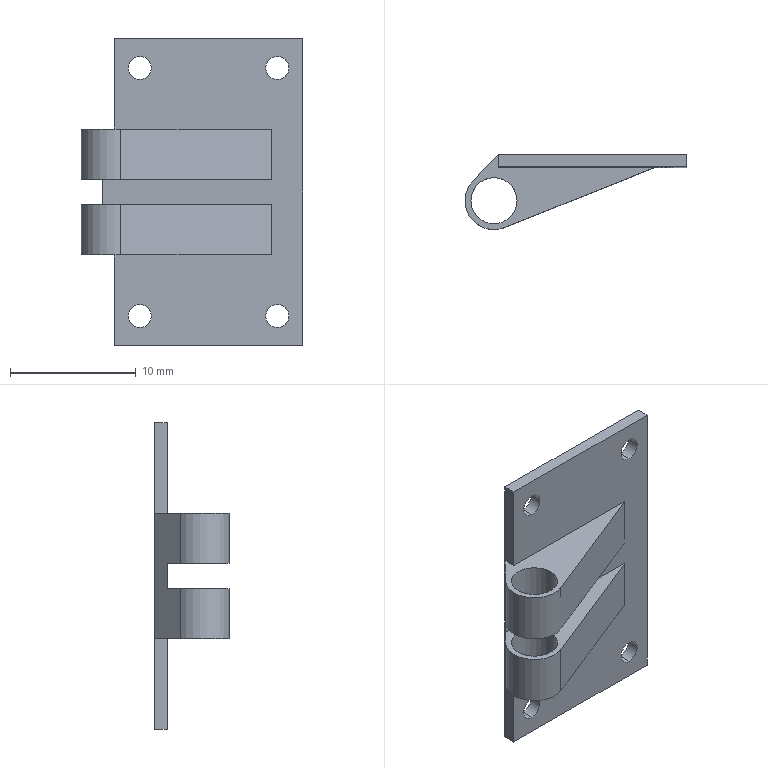Part | SolidWorks | features BaseBody 1 | 1 solid | 28 faces | box 17.607 x 5.957 x 24.289 mm | volume 605.772 mm3 | cylinder 14 | plane 14 | commonest cylinder face diameters 1.828 x8 3.663 x4 4.588 x2
STEP:
#1=CARTESIAN_POINT('',(185.615,42.862,-8.93));
#2=VERTEX_POINT('',#1);
#3=CARTESIAN_POINT('',(185.615,42.862,-10.758));
#4=VERTEX_POINT('',#3);
#5=CARTESIAN_POINT('',(185.615,42.862,-9.844));
#6=DIRECTION('',(0.,-1.,0.));
#7=DIRECTION('',(0.,0.,-1.));
#8=AXIS2_PLACEMENT_3D('',#5,#6,#7);
#9=CIRCLE('',#8,0.9139);
#10=EDGE_CURVE('',#2,#4,#9,.T.);
#11=ORIENTED_EDGE('',*,*,#10,.F.);
#12=CARTESIAN_POINT('',(185.615,41.862,-8.93));
#13=VERTEX_POINT('',#12);
#14=CARTESIAN_POINT('',(185.615,42.862,-8.93));
#15=DIRECTION('',(0.,-1.,0.));
#16=VECTOR('',#15,1000.);
#17=LINE('',#14,#16);
#18=EDGE_CURVE('',#2,#13,#17,.T.);
#19=ORIENTED_EDGE('',*,*,#18,.T.);
#20=CARTESIAN_POINT('',(185.615,41.862,-10.758));
#21=VERTEX_POINT('',#20);
#22=CARTESIAN_POINT('',(185.615,41.862,-9.844));
#23=DIRECTION('',(0.,1.,0.));
#24=DIRECTION('',(0.,0.,-1.));
#25=AXIS2_PLACEMENT_3D('',#22,#23,#24);
#26=CIRCLE('',#25,0.9139);
#27=EDGE_CURVE('',#21,#13,#26,.T.);
#28=ORIENTED_EDGE('',*,*,#27,.F.);
#29=CARTESIAN_POINT('',(185.615,42.862,-10.758));
#30=DIRECTION('',(0.,-1.,0.));
#31=VECTOR('',#30,1000.);
#32=LINE('',#29,#31);
#33=EDGE_CURVE('',#4,#21,#32,.T.);
#34=ORIENTED_EDGE('',*,*,#33,.F.);
#35=EDGE_LOOP('',(#11,#19,#28,#34));
#36=FACE_OUTER_BOUND('',#35,.T.);
#37=CARTESIAN_POINT('',(185.615,42.862,-9.844));
#38=DIRECTION('',(0.,-1.,0.));
#39=DIRECTION('',(0.,0.,-1.));
#40=AXIS2_PLACEMENT_3D('',#37,#38,#39);
#41=CYLINDRICAL_SURFACE('',#40,0.9139);
#42=ADVANCED_FACE('',(#36),#41,.F.);
#43=CARTESIAN_POINT('',(196.532,42.862,-8.93));
#44=VERTEX_POINT('',#43);
#45=CARTESIAN_POINT('',(196.532,42.862,-10.758));
#46=VERTEX_POINT('',#45);
#47=CARTESIAN_POINT('',(196.532,42.862,-9.844));
#48=DIRECTION('',(0.,-1.,0.));
#49=DIRECTION('',(0.,0.,-1.));
#50=AXIS2_PLACEMENT_3D('',#47,#48,#49);
#51=CIRCLE('',#50,0.9139);
#52=EDGE_CURVE('',#44,#46,#51,.T.);
#53=ORIENTED_EDGE('',*,*,#52,.F.);
#54=CARTESIAN_POINT('',(196.532,41.862,-8.93));
#55=VERTEX_POINT('',#54);
#56=CARTESIAN_POINT('',(196.532,42.862,-8.93));
#57=DIRECTION('',(0.,-1.,0.));
#58=VECTOR('',#57,1000.);
#59=LINE('',#56,#58);
#60=EDGE_CURVE('',#44,#55,#59,.T.);
#61=ORIENTED_EDGE('',*,*,#60,.T.);
#62=CARTESIAN_POINT('',(196.532,41.862,-10.758));
#63=VERTEX_POINT('',#62);
#64=CARTESIAN_POINT('',(196.532,41.862,-9.844));
#65=DIRECTION('',(0.,1.,0.));
#66=DIRECTION('',(0.,0.,-1.));
#67=AXIS2_PLACEMENT_3D('',#64,#65,#66);
#68=CIRCLE('',#67,0.9139);
#69=EDGE_CURVE('',#63,#55,#68,.T.);
#70=ORIENTED_EDGE('',*,*,#69,.F.);
#71=CARTESIAN_POINT('',(196.532,42.862,-10.758));
#72=DIRECTION('',(0.,-1.,0.));
#73=VECTOR('',#72,1000.);
#74=LINE('',#71,#73);
#75=EDGE_CURVE('',#46,#63,#74,.T.);
#76=ORIENTED_EDGE('',*,*,#75,.F.);
#77=EDGE_LOOP('',(#53,#61,#70,#76));
#78=FACE_OUTER_BOUND('',#77,.T.);
#79=CARTESIAN_POINT('',(196.532,42.862,-9.844));
#80=DIRECTION('',(0.,-1.,0.));
#81=DIRECTION('',(0.,0.,-1.));
#82=AXIS2_PLACEMENT_3D('',#79,#80,#81);
#83=CYLINDRICAL_SURFACE('',#82,0.9139);
#84=ADVANCED_FACE('',(#78),#83,.F.);
#85=CARTESIAN_POINT('',(196.532,42.862,10.758));
#86=VERTEX_POINT('',#85);
#87=CARTESIAN_POINT('',(196.532,42.862,8.93));
#88=VERTEX_POINT('',#87);
#89=CARTESIAN_POINT('',(196.532,42.862,9.844));
#90=DIRECTION('',(0.,-1.,0.));
#91=DIRECTION('',(0.,0.,-1.));
#92=AXIS2_PLACEMENT_3D('',#89,#90,#91);
#93=CIRCLE('',#92,0.9139);
#94=EDGE_CURVE('',#86,#88,#93,.T.);
#95=ORIENTED_EDGE('',*,*,#94,.F.);
#96=CARTESIAN_POINT('',(196.532,41.862,10.758));
#97=VERTEX_POINT('',#96);
#98=CARTESIAN_POINT('',(196.532,42.862,10.758));
#99=DIRECTION('',(0.,-1.,0.));
#100=VECTOR('',#99,1000.);
#101=LINE('',#98,#100);
#102=EDGE_CURVE('',#86,#97,#101,.T.);
#103=ORIENTED_EDGE('',*,*,#102,.T.);
#104=CARTESIAN_POINT('',(196.532,41.862,8.93));
#105=VERTEX_POINT('',#104);
#106=CARTESIAN_POINT('',(196.532,41.862,9.844));
#107=DIRECTION('',(0.,1.,0.));
#108=DIRECTION('',(0.,0.,-1.));
#109=AXIS2_PLACEMENT_3D('',#106,#107,#108);
#110=CIRCLE('',#109,0.9139);
#111=EDGE_CURVE('',#105,#97,#110,.T.);
#112=ORIENTED_EDGE('',*,*,#111,.F.);
#113=CARTESIAN_POINT('',(196.532,42.862,8.93));
#114=DIRECTION('',(0.,-1.,0.));
#115=VECTOR('',#114,1000.);
#116=LINE('',#113,#115);
#117=EDGE_CURVE('',#88,#105,#116,.T.);
#118=ORIENTED_EDGE('',*,*,#117,.F.);
#119=EDGE_LOOP('',(#95,#103,#112,#118));
#120=FACE_OUTER_BOUND('',#119,.T.);
#121=CARTESIAN_POINT('',(196.532,42.862,9.844));
#122=DIRECTION('',(0.,-1.,0.));
#123=DIRECTION('',(0.,0.,-1.));
#124=AXIS2_PLACEMENT_3D('',#121,#122,#123);
#125=CYLINDRICAL_SURFACE('',#124,0.9139);
#126=ADVANCED_FACE('',(#120),#125,.F.);
#127=CARTESIAN_POINT('',(185.615,42.862,10.758));
#128=VERTEX_POINT('',#127);
#129=CARTESIAN_POINT('',(185.615,42.862,8.93));
#130=VERTEX_POINT('',#129);
#131=CARTESIAN_POINT('',(185.615,42.862,9.844));
#132=DIRECTION('',(0.,-1.,0.));
#133=DIRECTION('',(0.,0.,-1.));
#134=AXIS2_PLACEMENT_3D('',#131,#132,#133);
#135=CIRCLE('',#134,0.9139);
#136=EDGE_CURVE('',#128,#130,#135,.T.);
#137=ORIENTED_EDGE('',*,*,#136,.F.);
#138=CARTESIAN_POINT('',(185.615,41.862,10.758));
#139=VERTEX_POINT('',#138);
#140=CARTESIAN_POINT('',(185.615,42.862,10.758));
#141=DIRECTION('',(0.,-1.,0.));
#142=VECTOR('',#141,1000.);
#143=LINE('',#140,#142);
#144=EDGE_CURVE('',#128,#139,#143,.T.);
#145=ORIENTED_EDGE('',*,*,#144,.T.);
#146=CARTESIAN_POINT('',(185.615,41.862,8.93));
#147=VERTEX_POINT('',#146);
#148=CARTESIAN_POINT('',(185.615,41.862,9.844));
#149=DIRECTION('',(0.,1.,0.));
#150=DIRECTION('',(0.,0.,-1.));
#151=AXIS2_PLACEMENT_3D('',#148,#149,#150);
#152=CIRCLE('',#151,0.9139);
#153=EDGE_CURVE('',#147,#139,#152,.T.);
#154=ORIENTED_EDGE('',*,*,#153,.F.);
#155=CARTESIAN_POINT('',(185.615,42.862,8.93));
#156=DIRECTION('',(0.,-1.,0.));
#157=VECTOR('',#156,1000.);
#158=LINE('',#155,#157);
#159=EDGE_CURVE('',#130,#147,#158,.T.);
#160=ORIENTED_EDGE('',*,*,#159,.F.);
#161=EDGE_LOOP('',(#137,#145,#154,#160));
#162=FACE_OUTER_BOUND('',#161,.T.);
#163=CARTESIAN_POINT('',(185.615,42.862,9.844));
#164=DIRECTION('',(0.,-1.,0.));
#165=DIRECTION('',(0.,0.,-1.));
#166=AXIS2_PLACEMENT_3D('',#163,#164,#165);
#167=CYLINDRICAL_SURFACE('',#166,0.9139);
#168=ADVANCED_FACE('',(#162),#167,.F.);
#169=CARTESIAN_POINT('',(185.074,39.199,-5.));
#170=VERTEX_POINT('',#169);
#171=CARTESIAN_POINT('',(181.411,39.199,-5.));
#172=VERTEX_POINT('',#171);
#173=CARTESIAN_POINT('',(183.243,39.199,-5.));
#174=DIRECTION('',(0.,0.,-1.));
#175=DIRECTION('',(1.,0.,0.));
#176=AXIS2_PLACEMENT_3D('',#173,#174,#175);
#177=CIRCLE('',#176,1.832);
#178=EDGE_CURVE('',#170,#172,#177,.T.);
#179=ORIENTED_EDGE('',*,*,#178,.T.);
#180=CARTESIAN_POINT('',(181.411,39.199,-1.));
#181=VERTEX_POINT('',#180);
#182=CARTESIAN_POINT('',(181.411,39.199,0.));
#183=DIRECTION('',(0.,0.,1.));
#184=VECTOR('',#183,1000.);
#185=LINE('',#182,#184);
#186=EDGE_CURVE('',#172,#181,#185,.T.);
#187=ORIENTED_EDGE('',*,*,#186,.T.);
#188=CARTESIAN_POINT('',(185.074,39.199,-1.));
#189=VERTEX_POINT('',#188);
#190=CARTESIAN_POINT('',(183.243,39.199,-1.));
#191=DIRECTION('',(0.,0.,1.));
#192=DIRECTION('',(1.,0.,0.));
#193=AXIS2_PLACEMENT_3D('',#190,#191,#192);
#194=CIRCLE('',#193,1.832);
#195=EDGE_CURVE('',#181,#189,#194,.T.);
#196=ORIENTED_EDGE('',*,*,#195,.T.);
#197=CARTESIAN_POINT('',(185.074,39.199,0.));
#198=DIRECTION('',(0.,0.,1.));
#199=VECTOR('',#198,1000.);
#200=LINE('',#197,#199);
#201=EDGE_CURVE('',#170,#189,#200,.T.);
#202=ORIENTED_EDGE('',*,*,#201,.F.);
#203=EDGE_LOOP('',(#179,#187,#196,#202));
#204=FACE_OUTER_BOUND('',#203,.T.);
#205=CARTESIAN_POINT('',(183.243,39.199,0.));
#206=DIRECTION('',(0.,0.,1.));
#207=DIRECTION('',(1.,0.,0.));
#208=AXIS2_PLACEMENT_3D('',#205,#206,#207);
#209=CYLINDRICAL_SURFACE('',#208,1.832);
#210=ADVANCED_FACE('',(#204),#209,.F.);
#211=CARTESIAN_POINT('',(185.074,39.199,1.));
#212=VERTEX_POINT('',#211);
#213=CARTESIAN_POINT('',(181.411,39.199,1.));
#214=VERTEX_POINT('',#213);
#215=CARTESIAN_POINT('',(183.243,39.199,1.));
#216=DIRECTION('',(0.,0.,-1.));
#217=DIRECTION('',(1.,0.,0.));
#218=AXIS2_PLACEMENT_3D('',#215,#216,#217);
#219=CIRCLE('',#218,1.832);
#220=EDGE_CURVE('',#212,#214,#219,.T.);
#221=ORIENTED_EDGE('',*,*,#220,.T.);
#222=CARTESIAN_POINT('',(181.411,39.199,5.));
#223=VERTEX_POINT('',#222);
#224=CARTESIAN_POINT('',(181.411,39.199,0.));
#225=DIRECTION('',(0.,0.,1.));
#226=VECTOR('',#225,1000.);
#227=LINE('',#224,#226);
#228=EDGE_CURVE('',#214,#223,#227,.T.);
#229=ORIENTED_EDGE('',*,*,#228,.T.);
#230=CARTESIAN_POINT('',(185.074,39.199,5.));
#231=VERTEX_POINT('',#230);
#232=CARTESIAN_POINT('',(183.243,39.199,5.));
#233=DIRECTION('',(0.,0.,-1.));
#234=DIRECTION('',(1.,0.,0.));
#235=AXIS2_PLACEMENT_3D('',#232,#233,#234);
#236=CIRCLE('',#235,1.832);
#237=EDGE_CURVE('',#231,#223,#236,.T.);
#238=ORIENTED_EDGE('',*,*,#237,.F.);
#239=CARTESIAN_POINT('',(185.074,39.199,0.));
#240=DIRECTION('',(0.,0.,1.));
#241=VECTOR('',#240,1000.);
#242=LINE('',#239,#241);
#243=EDGE_CURVE('',#212,#231,#242,.T.);
#244=ORIENTED_EDGE('',*,*,#243,.F.);
#245=EDGE_LOOP('',(#221,#229,#238,#244));
#246=FACE_OUTER_BOUND('',#245,.T.);
#247=CARTESIAN_POINT('',(183.243,39.199,0.));
#248=DIRECTION('',(0.,0.,1.));
#249=DIRECTION('',(1.,0.,0.));
#250=AXIS2_PLACEMENT_3D('',#247,#248,#249);
#251=CYLINDRICAL_SURFACE('',#250,1.832);
#252=ADVANCED_FACE('',(#246),#251,.F.);
#253=CARTESIAN_POINT('',(185.615,42.862,-9.844));
#254=DIRECTION('',(0.,-1.,0.));
#255=DIRECTION('',(0.,0.,-1.));
#256=AXIS2_PLACEMENT_3D('',#253,#254,#255);
#257=CIRCLE('',#256,0.9139);
#258=EDGE_CURVE('',#4,#2,#257,.T.);
#259=ORIENTED_EDGE('',*,*,#258,.T.);
#260=ORIENTED_EDGE('',*,*,#10,.T.);
#261=EDGE_LOOP('',(#259,#260));
#262=FACE_BOUND('',#261,.T.);
#263=CARTESIAN_POINT('',(196.532,42.862,-9.844));
#264=DIRECTION('',(0.,-1.,0.));
#265=DIRECTION('',(0.,0.,-1.));
#266=AXIS2_PLACEMENT_3D('',#263,#264,#265);
#267=CIRCLE('',#266,0.9139);
#268=EDGE_CURVE('',#46,#44,#267,.T.);
#269=ORIENTED_EDGE('',*,*,#268,.T.);
#270=ORIENTED_EDGE('',*,*,#52,.T.);
#271=EDGE_LOOP('',(#269,#270));
#272=FACE_BOUND('',#271,.T.);
#273=CARTESIAN_POINT('',(196.532,42.862,9.844));
#274=DIRECTION('',(0.,-1.,0.));
#275=DIRECTION('',(0.,0.,-1.));
#276=AXIS2_PLACEMENT_3D('',#273,#274,#275);
#277=CIRCLE('',#276,0.9139);
#278=EDGE_CURVE('',#88,#86,#277,.T.);
#279=ORIENTED_EDGE('',*,*,#278,.T.);
#280=ORIENTED_EDGE('',*,*,#94,.T.);
#281=EDGE_LOOP('',(#279,#280));
#282=FACE_BOUND('',#281,.T.);
#283=CARTESIAN_POINT('',(185.615,42.862,9.844));
#284=DIRECTION('',(0.,-1.,0.));
#285=DIRECTION('',(0.,0.,-1.));
#286=AXIS2_PLACEMENT_3D('',#283,#284,#285);
#287=CIRCLE('',#286,0.9139);
#288=EDGE_CURVE('',#130,#128,#287,.T.);
#289=ORIENTED_EDGE('',*,*,#288,.T.);
#290=ORIENTED_EDGE('',*,*,#136,.T.);
#291=EDGE_LOOP('',(#289,#290));
#292=FACE_BOUND('',#291,.T.);
#293=CARTESIAN_POINT('',(198.556,42.862,-12.144));
#294=VERTEX_POINT('',#293);
#295=CARTESIAN_POINT('',(183.591,42.862,-12.144));
#296=VERTEX_POINT('',#295);
#297=CARTESIAN_POINT('',(198.556,42.862,-12.144));
#298=DIRECTION('',(-1.,0.,0.));
#299=VECTOR('',#298,1000.);
#300=LINE('',#297,#299);
#301=EDGE_CURVE('',#294,#296,#300,.T.);
#302=ORIENTED_EDGE('',*,*,#301,.T.);
#303=CARTESIAN_POINT('',(183.591,42.862,-5.));
#304=VERTEX_POINT('',#303);
#305=CARTESIAN_POINT('',(183.591,42.862,0.));
#306=DIRECTION('',(0.,0.,1.));
#307=VECTOR('',#306,1000.);
#308=LINE('',#305,#307);
#309=EDGE_CURVE('',#296,#304,#308,.T.);
#310=ORIENTED_EDGE('',*,*,#309,.T.);
#311=CARTESIAN_POINT('',(183.591,42.862,5.));
#312=VERTEX_POINT('',#311);
#313=CARTESIAN_POINT('',(183.591,42.862,0.));
#314=DIRECTION('',(0.,0.,1.));
#315=VECTOR('',#314,1000.);
#316=LINE('',#313,#315);
#317=EDGE_CURVE('',#304,#312,#316,.T.);
#318=ORIENTED_EDGE('',*,*,#317,.T.);
#319=CARTESIAN_POINT('',(183.591,42.862,12.144));
#320=VERTEX_POINT('',#319);
#321=CARTESIAN_POINT('',(183.591,42.862,0.));
#322=DIRECTION('',(0.,0.,1.));
#323=VECTOR('',#322,1000.);
#324=LINE('',#321,#323);
#325=EDGE_CURVE('',#312,#320,#324,.T.);
#326=ORIENTED_EDGE('',*,*,#325,.T.);
#327=CARTESIAN_POINT('',(198.556,42.862,12.144));
#328=VERTEX_POINT('',#327);
#329=CARTESIAN_POINT('',(198.556,42.862,12.144));
#330=DIRECTION('',(1.,0.,0.));
#331=VECTOR('',#330,1000.);
#332=LINE('',#329,#331);
#333=EDGE_CURVE('',#320,#328,#332,.T.);
#334=ORIENTED_EDGE('',*,*,#333,.T.);
#335=CARTESIAN_POINT('',(198.556,42.862,0.));
#336=DIRECTION('',(0.,0.,-1.));
#337=VECTOR('',#336,1000.);
#338=LINE('',#335,#337);
#339=EDGE_CURVE('',#328,#294,#338,.T.);
#340=ORIENTED_EDGE('',*,*,#339,.T.);
#341=EDGE_LOOP('',(#302,#310,#318,#326,#334,#340));
#342=FACE_OUTER_BOUND('',#341,.T.);
#343=CARTESIAN_POINT('',(198.556,42.862,0.));
#344=DIRECTION('',(0.,1.,0.));
#345=DIRECTION('',(0.,0.,1.));
#346=AXIS2_PLACEMENT_3D('',#343,#344,#345);
#347=PLANE('',#346);
#348=ADVANCED_FACE('',(#262,#272,#282,#292,#342),#347,.T.);
#349=ORIENTED_EDGE('',*,*,#18,.F.);
#350=ORIENTED_EDGE('',*,*,#258,.F.);
#351=ORIENTED_EDGE('',*,*,#33,.T.);
#352=CARTESIAN_POINT('',(185.615,41.862,-9.844));
#353=DIRECTION('',(0.,1.,0.));
#354=DIRECTION('',(0.,0.,-1.));
#355=AXIS2_PLACEMENT_3D('',#352,#353,#354);
#356=CIRCLE('',#355,0.9139);
#357=EDGE_CURVE('',#13,#21,#356,.T.);
#358=ORIENTED_EDGE('',*,*,#357,.F.);
#359=EDGE_LOOP('',(#349,#350,#351,#358));
#360=FACE_OUTER_BOUND('',#359,.T.);
#361=CARTESIAN_POINT('',(185.615,42.862,-9.844));
#362=DIRECTION('',(0.,-1.,0.));
#363=DIRECTION('',(0.,0.,-1.));
#364=AXIS2_PLACEMENT_3D('',#361,#362,#363);
#365=CYLINDRICAL_SURFACE('',#364,0.9139);
#366=ADVANCED_FACE('',(#360),#365,.F.);
#367=ORIENTED_EDGE('',*,*,#60,.F.);
#368=ORIENTED_EDGE('',*,*,#268,.F.);
#369=ORIENTED_EDGE('',*,*,#75,.T.);
#370=CARTESIAN_POINT('',(196.532,41.862,-9.844));
#371=DIRECTION('',(0.,1.,0.));
#372=DIRECTION('',(0.,0.,-1.));
#373=AXIS2_PLACEMENT_3D('',#370,#371,#372);
#374=CIRCLE('',#373,0.9139);
#375=EDGE_CURVE('',#55,#63,#374,.T.);
#376=ORIENTED_EDGE('',*,*,#375,.F.);
#377=EDGE_LOOP('',(#367,#368,#369,#376));
#378=FACE_OUTER_BOUND('',#377,.T.);
#379=CARTESIAN_POINT('',(196.532,42.862,-9.844));
#380=DIRECTION('',(0.,-1.,0.));
#381=DIRECTION('',(0.,0.,-1.));
#382=AXIS2_PLACEMENT_3D('',#379,#380,#381);
#383=CYLINDRICAL_SURFACE('',#382,0.9139);
#384=ADVANCED_FACE('',(#378),#383,.F.);
#385=ORIENTED_EDGE('',*,*,#102,.F.);
#386=ORIENTED_EDGE('',*,*,#278,.F.);
#387=ORIENTED_EDGE('',*,*,#117,.T.);
#388=CARTESIAN_POINT('',(196.532,41.862,9.844));
#389=DIRECTION('',(0.,1.,0.));
#390=DIRECTION('',(0.,0.,-1.));
#391=AXIS2_PLACEMENT_3D('',#388,#389,#390);
#392=CIRCLE('',#391,0.9139);
#393=EDGE_CURVE('',#97,#105,#392,.T.);
#394=ORIENTED_EDGE('',*,*,#393,.F.);
#395=EDGE_LOOP('',(#385,#386,#387,#394));
#396=FACE_OUTER_BOUND('',#395,.T.);
#397=CARTESIAN_POINT('',(196.532,42.862,9.844));
#398=DIRECTION('',(0.,-1.,0.));
#399=DIRECTION('',(0.,0.,-1.));
#400=AXIS2_PLACEMENT_3D('',#397,#398,#399);
#401=CYLINDRICAL_SURFACE('',#400,0.9139);
#402=ADVANCED_FACE('',(#396),#401,.F.);
#403=ORIENTED_EDGE('',*,*,#144,.F.);
#404=ORIENTED_EDGE('',*,*,#288,.F.);
#405=ORIENTED_EDGE('',*,*,#159,.T.);
#406=CARTESIAN_POINT('',(185.615,41.862,9.844));
#407=DIRECTION('',(0.,1.,0.));
#408=DIRECTION('',(0.,0.,-1.));
#409=AXIS2_PLACEMENT_3D('',#406,#407,#408);
#410=CIRCLE('',#409,0.9139);
#411=EDGE_CURVE('',#139,#147,#410,.T.);
#412=ORIENTED_EDGE('',*,*,#411,.F.);
#413=EDGE_LOOP('',(#403,#404,#405,#412));
#414=FACE_OUTER_BOUND('',#413,.T.);
#415=CARTESIAN_POINT('',(185.615,42.862,9.844));
#416=DIRECTION('',(0.,-1.,0.));
#417=DIRECTION('',(0.,0.,-1.));
#418=AXIS2_PLACEMENT_3D('',#415,#416,#417);
#419=CYLINDRICAL_SURFACE('',#418,0.9139);
#420=ADVANCED_FACE('',(#414),#419,.F.);
#421=CARTESIAN_POINT('',(183.591,41.862,-12.144));
#422=VERTEX_POINT('',#421);
#423=CARTESIAN_POINT('',(183.591,42.862,-12.144));
#424=DIRECTION('',(0.,-1.,0.));
#425=VECTOR('',#424,1000.);
#426=LINE('',#423,#425);
#427=EDGE_CURVE('',#296,#422,#426,.T.);
#428=ORIENTED_EDGE('',*,*,#427,.T.);
#429=CARTESIAN_POINT('',(183.591,41.862,-5.));
#430=VERTEX_POINT('',#429);
#431=CARTESIAN_POINT('',(183.591,41.862,12.144));
#432=DIRECTION('',(0.,0.,1.));
#433=VECTOR('',#432,1000.);
#434=LINE('',#431,#433);
#435=EDGE_CURVE('',#422,#430,#434,.T.);
#436=ORIENTED_EDGE('',*,*,#435,.T.);
#437=CARTESIAN_POINT('',(183.591,39.884,-5.));
#438=DIRECTION('',(0.,1.,0.));
#439=VECTOR('',#438,1000.);
#440=LINE('',#437,#439);
#441=EDGE_CURVE('',#430,#304,#440,.T.);
#442=ORIENTED_EDGE('',*,*,#441,.T.);
#443=ORIENTED_EDGE('',*,*,#309,.F.);
#444=EDGE_LOOP('',(#428,#436,#442,#443));
#445=FACE_OUTER_BOUND('',#444,.T.);
#446=CARTESIAN_POINT('',(183.591,42.862,12.144));
#447=DIRECTION('',(-1.,0.,0.));
#448=DIRECTION('',(0.,0.,1.));
#449=AXIS2_PLACEMENT_3D('',#446,#447,#448);
#450=PLANE('',#449);
#451=ADVANCED_FACE('',(#445),#450,.T.);
#452=CARTESIAN_POINT('',(198.556,41.862,-12.144));
#453=VERTEX_POINT('',#452);
#454=CARTESIAN_POINT('',(183.591,41.862,-12.144));
#455=DIRECTION('',(-1.,0.,0.));
#456=VECTOR('',#455,1000.);
#457=LINE('',#454,#456);
#458=EDGE_CURVE('',#453,#422,#457,.T.);
#459=ORIENTED_EDGE('',*,*,#458,.T.);
#460=ORIENTED_EDGE('',*,*,#427,.F.);
#461=ORIENTED_EDGE('',*,*,#301,.F.);
#462=CARTESIAN_POINT('',(198.556,42.862,-12.144));
#463=DIRECTION('',(0.,-1.,0.));
#464=VECTOR('',#463,1000.);
#465=LINE('',#462,#464);
#466=EDGE_CURVE('',#294,#453,#465,.T.);
#467=ORIENTED_EDGE('',*,*,#466,.T.);
#468=EDGE_LOOP('',(#459,#460,#461,#467));
#469=FACE_OUTER_BOUND('',#468,.T.);
#470=CARTESIAN_POINT('',(183.591,42.862,-12.144));
#471=DIRECTION('',(0.,0.,-1.));
#472=DIRECTION('',(-1.,0.,0.));
#473=AXIS2_PLACEMENT_3D('',#470,#471,#472);
#474=PLANE('',#473);
#475=ADVANCED_FACE('',(#469),#474,.T.);
#476=CARTESIAN_POINT('',(198.556,41.862,12.144));
#477=VERTEX_POINT('',#476);
#478=CARTESIAN_POINT('',(198.556,41.862,-12.144));
#479=DIRECTION('',(0.,0.,-1.));
#480=VECTOR('',#479,1000.);
#481=LINE('',#478,#480);
#482=EDGE_CURVE('',#477,#453,#481,.T.);
#483=ORIENTED_EDGE('',*,*,#482,.T.);
#484=ORIENTED_EDGE('',*,*,#466,.F.);
#485=ORIENTED_EDGE('',*,*,#339,.F.);
#486=CARTESIAN_POINT('',(198.556,42.862,12.144));
#487=DIRECTION('',(0.,-1.,0.));
#488=VECTOR('',#487,1000.);
#489=LINE('',#486,#488);
#490=EDGE_CURVE('',#328,#477,#489,.T.);
#491=ORIENTED_EDGE('',*,*,#490,.T.);
#492=EDGE_LOOP('',(#483,#484,#485,#491));
#493=FACE_OUTER_BOUND('',#492,.T.);
#494=CARTESIAN_POINT('',(198.556,42.862,-12.144));
#495=DIRECTION('',(1.,0.,0.));
#496=DIRECTION('',(0.,0.,-1.));
#497=AXIS2_PLACEMENT_3D('',#494,#495,#496);
#498=PLANE('',#497);
#499=ADVANCED_FACE('',(#493),#498,.T.);
#500=CARTESIAN_POINT('',(183.591,41.862,12.144));
#501=VERTEX_POINT('',#500);
#502=CARTESIAN_POINT('',(198.556,41.862,12.144));
#503=DIRECTION('',(1.,0.,0.));
#504=VECTOR('',#503,1000.);
#505=LINE('',#502,#504);
#506=EDGE_CURVE('',#501,#477,#505,.T.);
#507=ORIENTED_EDGE('',*,*,#506,.T.);
#508=ORIENTED_EDGE('',*,*,#490,.F.);
#509=ORIENTED_EDGE('',*,*,#333,.F.);
#510=CARTESIAN_POINT('',(183.591,42.862,12.144));
#511=DIRECTION('',(0.,-1.,0.));
#512=VECTOR('',#511,1000.);
#513=LINE('',#510,#512);
#514=EDGE_CURVE('',#320,#501,#513,.T.);
#515=ORIENTED_EDGE('',*,*,#514,.T.);
#516=EDGE_LOOP('',(#507,#508,#509,#515));
#517=FACE_OUTER_BOUND('',#516,.T.);
#518=CARTESIAN_POINT('',(198.556,42.862,12.144));
#519=DIRECTION('',(0.,0.,1.));
#520=DIRECTION('',(1.,0.,0.));
#521=AXIS2_PLACEMENT_3D('',#518,#519,#520);
#522=PLANE('',#521);
#523=ADVANCED_FACE('',(#517),#522,.T.);
#524=ORIENTED_EDGE('',*,*,#514,.F.);
#525=ORIENTED_EDGE('',*,*,#325,.F.);
#526=CARTESIAN_POINT('',(183.591,41.862,5.));
#527=VERTEX_POINT('',#526);
#528=CARTESIAN_POINT('',(183.591,39.884,5.));
#529=DIRECTION('',(0.,1.,0.));
#530=VECTOR('',#529,1000.);
#531=LINE('',#528,#530);
#532=EDGE_CURVE('',#527,#312,#531,.T.);
#533=ORIENTED_EDGE('',*,*,#532,.F.);
#534=CARTESIAN_POINT('',(183.591,41.862,12.144));
#535=DIRECTION('',(0.,0.,1.));
#536=VECTOR('',#535,1000.);
#537=LINE('',#534,#536);
#538=EDGE_CURVE('',#527,#501,#537,.T.);
#539=ORIENTED_EDGE('',*,*,#538,.T.);
#540=EDGE_LOOP('',(#524,#525,#533,#539));
#541=FACE_OUTER_BOUND('',#540,.T.);
#542=CARTESIAN_POINT('',(183.591,42.862,12.144));
#543=DIRECTION('',(-1.,0.,0.));
#544=DIRECTION('',(0.,0.,1.));
#545=AXIS2_PLACEMENT_3D('',#542,#543,#544);
#546=PLANE('',#545);
#547=ADVANCED_FACE('',(#541),#546,.T.);
#548=CARTESIAN_POINT('',(181.592,40.793,-5.));
#549=VERTEX_POINT('',#548);
#550=CARTESIAN_POINT('',(183.591,42.862,-5.));
#551=DIRECTION('',(-0.6946,-0.7194,0.));
#552=VECTOR('',#551,1000.);
#553=LINE('',#550,#552);
#554=EDGE_CURVE('',#304,#549,#553,.T.);
#555=ORIENTED_EDGE('',*,*,#554,.T.);
#556=CARTESIAN_POINT('',(181.592,40.793,-1.));
#557=VERTEX_POINT('',#556);
#558=CARTESIAN_POINT('',(181.592,40.793,0.));
#559=DIRECTION('',(0.,0.,1.));
#560=VECTOR('',#559,1000.);
#561=LINE('',#558,#560);
#562=EDGE_CURVE('',#549,#557,#561,.T.);
#563=ORIENTED_EDGE('',*,*,#562,.T.);
#564=CARTESIAN_POINT('',(182.626,41.863,-1.));
#565=VERTEX_POINT('',#564);
#566=CARTESIAN_POINT('',(181.592,40.793,-1.));
#567=DIRECTION('',(0.6946,0.7194,0.));
#568=VECTOR('',#567,1000.);
#569=LINE('',#566,#568);
#570=EDGE_CURVE('',#557,#565,#569,.T.);
#571=ORIENTED_EDGE('',*,*,#570,.T.);
#572=CARTESIAN_POINT('',(182.626,41.862,1.));
#573=VERTEX_POINT('',#572);
#574=CARTESIAN_POINT('',(182.626,41.863,0.));
#575=DIRECTION('',(0.,0.,1.));
#576=VECTOR('',#575,1000.);
#577=LINE('',#574,#576);
#578=EDGE_CURVE('',#565,#573,#577,.T.);
#579=ORIENTED_EDGE('',*,*,#578,.T.);
#580=CARTESIAN_POINT('',(181.592,40.793,1.));
#581=VERTEX_POINT('',#580);
#582=CARTESIAN_POINT('',(182.626,41.862,1.));
#583=DIRECTION('',(-0.6946,-0.7194,0.));
#584=VECTOR('',#583,1000.);
#585=LINE('',#582,#584);
#586=EDGE_CURVE('',#573,#581,#585,.T.);
#587=ORIENTED_EDGE('',*,*,#586,.T.);
#588=CARTESIAN_POINT('',(181.592,40.793,5.));
#589=VERTEX_POINT('',#588);
#590=CARTESIAN_POINT('',(181.592,40.793,0.));
#591=DIRECTION('',(0.,0.,1.));
#592=VECTOR('',#591,1000.);
#593=LINE('',#590,#592);
#594=EDGE_CURVE('',#581,#589,#593,.T.);
#595=ORIENTED_EDGE('',*,*,#594,.T.);
#596=CARTESIAN_POINT('',(183.591,42.862,5.));
#597=DIRECTION('',(0.6946,0.7194,0.));
#598=VECTOR('',#597,1000.);
#599=LINE('',#596,#598);
#600=EDGE_CURVE('',#589,#312,#599,.T.);
#601=ORIENTED_EDGE('',*,*,#600,.T.);
#602=ORIENTED_EDGE('',*,*,#317,.F.);
#603=EDGE_LOOP('',(#555,#563,#571,#579,#587,#595,#601,#602));
#604=FACE_OUTER_BOUND('',#603,.T.);
#605=CARTESIAN_POINT('',(183.591,42.862,0.));
#606=DIRECTION('',(-0.7194,0.6946,0.));
#607=DIRECTION('',(-0.6946,-0.7194,0.));
#608=AXIS2_PLACEMENT_3D('',#605,#606,#607);
#609=PLANE('',#608);
#610=ADVANCED_FACE('',(#604),#609,.T.);
#611=ORIENTED_EDGE('',*,*,#27,.T.);
#612=ORIENTED_EDGE('',*,*,#357,.T.);
#613=EDGE_LOOP('',(#611,#612));
#614=FACE_BOUND('',#613,.T.);
#615=ORIENTED_EDGE('',*,*,#69,.T.);
#616=ORIENTED_EDGE('',*,*,#375,.T.);
#617=EDGE_LOOP('',(#615,#616));
#618=FACE_BOUND('',#617,.T.);
#619=ORIENTED_EDGE('',*,*,#111,.T.);
#620=ORIENTED_EDGE('',*,*,#393,.T.);
#621=EDGE_LOOP('',(#619,#620));
#622=FACE_BOUND('',#621,.T.);
#623=ORIENTED_EDGE('',*,*,#153,.T.);
#624=ORIENTED_EDGE('',*,*,#411,.T.);
#625=EDGE_LOOP('',(#623,#624));
#626=FACE_BOUND('',#625,.T.);
#627=CARTESIAN_POINT('',(196.06,41.862,-5.));
#628=VERTEX_POINT('',#627);
#629=CARTESIAN_POINT('',(191.074,41.862,-5.));
#630=DIRECTION('',(1.,0.,0.));
#631=VECTOR('',#630,1000.);
#632=LINE('',#629,#631);
#633=EDGE_CURVE('',#430,#628,#632,.T.);
#634=ORIENTED_EDGE('',*,*,#633,.F.);
#635=ORIENTED_EDGE('',*,*,#435,.F.);
#636=ORIENTED_EDGE('',*,*,#458,.F.);
#637=ORIENTED_EDGE('',*,*,#482,.F.);
#638=ORIENTED_EDGE('',*,*,#506,.F.);
#639=ORIENTED_EDGE('',*,*,#538,.F.);
#640=CARTESIAN_POINT('',(196.06,41.862,5.));
#641=VERTEX_POINT('',#640);
#642=CARTESIAN_POINT('',(191.074,41.862,5.));
#643=DIRECTION('',(-1.,0.,0.));
#644=VECTOR('',#643,1000.);
#645=LINE('',#642,#644);
#646=EDGE_CURVE('',#641,#527,#645,.T.);
#647=ORIENTED_EDGE('',*,*,#646,.F.);
#648=CARTESIAN_POINT('',(196.06,41.862,1.));
#649=VERTEX_POINT('',#648);
#650=CARTESIAN_POINT('',(196.06,41.862,0.));
#651=DIRECTION('',(0.,0.,1.));
#652=VECTOR('',#651,1000.);
#653=LINE('',#650,#652);
#654=EDGE_CURVE('',#649,#641,#653,.T.);
#655=ORIENTED_EDGE('',*,*,#654,.F.);
#656=CARTESIAN_POINT('',(191.074,41.862,1.));
#657=DIRECTION('',(1.,0.,0.));
#658=VECTOR('',#657,1000.);
#659=LINE('',#656,#658);
#660=EDGE_CURVE('',#573,#649,#659,.T.);
#661=ORIENTED_EDGE('',*,*,#660,.F.);
#662=ORIENTED_EDGE('',*,*,#578,.F.);
#663=CARTESIAN_POINT('',(196.06,41.862,-1.));
#664=VERTEX_POINT('',#663);
#665=CARTESIAN_POINT('',(191.074,41.862,-1.));
#666=DIRECTION('',(-1.,0.,0.));
#667=VECTOR('',#666,1000.);
#668=LINE('',#665,#667);
#669=EDGE_CURVE('',#664,#565,#668,.T.);
#670=ORIENTED_EDGE('',*,*,#669,.F.);
#671=CARTESIAN_POINT('',(196.06,41.862,0.));
#672=DIRECTION('',(0.,0.,1.));
#673=VECTOR('',#672,1000.);
#674=LINE('',#671,#673);
#675=EDGE_CURVE('',#628,#664,#674,.T.);
#676=ORIENTED_EDGE('',*,*,#675,.F.);
#677=EDGE_LOOP('',(#634,#635,#636,#637,#638,#639,#647,#655,#661,#662,#670,#676));
#678=FACE_OUTER_BOUND('',#677,.T.);
#679=CARTESIAN_POINT('',(191.074,41.862,0.));
#680=DIRECTION('',(0.,1.,0.));
#681=DIRECTION('',(0.,0.,1.));
#682=AXIS2_PLACEMENT_3D('',#679,#680,#681);
#683=PLANE('',#682);
#684=ADVANCED_FACE('',(#614,#618,#622,#626,#678),#683,.F.);
#685=CARTESIAN_POINT('',(184.096,37.07,-5.));
#686=VERTEX_POINT('',#685);
#687=CARTESIAN_POINT('',(183.243,39.199,-5.));
#688=DIRECTION('',(0.,0.,1.));
#689=DIRECTION('',(1.,0.,0.));
#690=AXIS2_PLACEMENT_3D('',#687,#688,#689);
#691=CIRCLE('',#690,2.294);
#692=EDGE_CURVE('',#549,#686,#691,.T.);
#693=ORIENTED_EDGE('',*,*,#692,.T.);
#694=CARTESIAN_POINT('',(184.096,37.07,-1.));
#695=VERTEX_POINT('',#694);
#696=CARTESIAN_POINT('',(184.096,37.07,0.));
#697=DIRECTION('',(0.,0.,1.));
#698=VECTOR('',#697,1000.);
#699=LINE('',#696,#698);
#700=EDGE_CURVE('',#686,#695,#699,.T.);
#701=ORIENTED_EDGE('',*,*,#700,.T.);
#702=CARTESIAN_POINT('',(183.243,39.199,-1.));
#703=DIRECTION('',(0.,0.,-1.));
#704=DIRECTION('',(1.,0.,0.));
#705=AXIS2_PLACEMENT_3D('',#702,#703,#704);
#706=CIRCLE('',#705,2.294);
#707=EDGE_CURVE('',#695,#557,#706,.T.);
#708=ORIENTED_EDGE('',*,*,#707,.T.);
#709=ORIENTED_EDGE('',*,*,#562,.F.);
#710=EDGE_LOOP('',(#693,#701,#708,#709));
#711=FACE_OUTER_BOUND('',#710,.T.);
#712=CARTESIAN_POINT('',(183.243,39.199,0.));
#713=DIRECTION('',(0.,0.,1.));
#714=DIRECTION('',(1.,0.,0.));
#715=AXIS2_PLACEMENT_3D('',#712,#713,#714);
#716=CYLINDRICAL_SURFACE('',#715,2.294);
#717=ADVANCED_FACE('',(#711),#716,.T.);
#718=ORIENTED_EDGE('',*,*,#178,.F.);
#719=CARTESIAN_POINT('',(183.243,39.199,-5.));
#720=DIRECTION('',(0.,0.,-1.));
#721=DIRECTION('',(1.,0.,0.));
#722=AXIS2_PLACEMENT_3D('',#719,#720,#721);
#723=CIRCLE('',#722,1.832);
#724=EDGE_CURVE('',#172,#170,#723,.T.);
#725=ORIENTED_EDGE('',*,*,#724,.F.);
#726=EDGE_LOOP('',(#718,#725));
#727=FACE_BOUND('',#726,.T.);
#728=CARTESIAN_POINT('',(184.096,37.07,-5.));
#729=DIRECTION('',(0.9283,0.3719,0.));
#730=VECTOR('',#729,1000.);
#731=LINE('',#728,#730);
#732=EDGE_CURVE('',#686,#628,#731,.T.);
#733=ORIENTED_EDGE('',*,*,#732,.F.);
#734=ORIENTED_EDGE('',*,*,#692,.F.);
#735=ORIENTED_EDGE('',*,*,#554,.F.);
#736=ORIENTED_EDGE('',*,*,#441,.F.);
#737=ORIENTED_EDGE('',*,*,#633,.T.);
#738=EDGE_LOOP('',(#733,#734,#735,#736,#737));
#739=FACE_OUTER_BOUND('',#738,.T.);
#740=CARTESIAN_POINT('',(189.752,39.884,-5.));
#741=DIRECTION('',(0.,0.,1.));
#742=DIRECTION('',(1.,0.,0.));
#743=AXIS2_PLACEMENT_3D('',#740,#741,#742);
#744=PLANE('',#743);
#745=ADVANCED_FACE('',(#727,#739),#744,.F.);
#746=ORIENTED_EDGE('',*,*,#237,.T.);
#747=CARTESIAN_POINT('',(183.243,39.199,5.));
#748=DIRECTION('',(0.,0.,-1.));
#749=DIRECTION('',(1.,0.,0.));
#750=AXIS2_PLACEMENT_3D('',#747,#748,#749);
#751=CIRCLE('',#750,1.832);
#752=EDGE_CURVE('',#223,#231,#751,.T.);
#753=ORIENTED_EDGE('',*,*,#752,.T.);
#754=EDGE_LOOP('',(#746,#753));
#755=FACE_BOUND('',#754,.T.);
#756=CARTESIAN_POINT('',(184.096,37.07,5.));
#757=VERTEX_POINT('',#756);
#758=CARTESIAN_POINT('',(183.243,39.199,5.));
#759=DIRECTION('',(0.,0.,1.));
#760=DIRECTION('',(1.,0.,0.));
#761=AXIS2_PLACEMENT_3D('',#758,#759,#760);
#762=CIRCLE('',#761,2.294);
#763=EDGE_CURVE('',#589,#757,#762,.T.);
#764=ORIENTED_EDGE('',*,*,#763,.T.);
#765=CARTESIAN_POINT('',(184.096,37.07,5.));
#766=DIRECTION('',(0.9283,0.3719,0.));
#767=VECTOR('',#766,1000.);
#768=LINE('',#765,#767);
#769=EDGE_CURVE('',#757,#641,#768,.T.);
#770=ORIENTED_EDGE('',*,*,#769,.T.);
#771=ORIENTED_EDGE('',*,*,#646,.T.);
#772=ORIENTED_EDGE('',*,*,#532,.T.);
#773=ORIENTED_EDGE('',*,*,#600,.F.);
#774=EDGE_LOOP('',(#764,#770,#771,#772,#773));
#775=FACE_OUTER_BOUND('',#774,.T.);
#776=CARTESIAN_POINT('',(189.752,39.884,5.));
#777=DIRECTION('',(0.,0.,1.));
#778=DIRECTION('',(1.,0.,0.));
#779=AXIS2_PLACEMENT_3D('',#776,#777,#778);
#780=PLANE('',#779);
#781=ADVANCED_FACE('',(#755,#775),#780,.T.);
#782=ORIENTED_EDGE('',*,*,#763,.F.);
#783=ORIENTED_EDGE('',*,*,#594,.F.);
#784=CARTESIAN_POINT('',(184.096,37.07,1.));
#785=VERTEX_POINT('',#784);
#786=CARTESIAN_POINT('',(183.243,39.199,1.));
#787=DIRECTION('',(0.,0.,1.));
#788=DIRECTION('',(1.,0.,0.));
#789=AXIS2_PLACEMENT_3D('',#786,#787,#788);
#790=CIRCLE('',#789,2.294);
#791=EDGE_CURVE('',#581,#785,#790,.T.);
#792=ORIENTED_EDGE('',*,*,#791,.T.);
#793=CARTESIAN_POINT('',(184.096,37.07,0.));
#794=DIRECTION('',(0.,0.,1.));
#795=VECTOR('',#794,1000.);
#796=LINE('',#793,#795);
#797=EDGE_CURVE('',#785,#757,#796,.T.);
#798=ORIENTED_EDGE('',*,*,#797,.T.);
#799=EDGE_LOOP('',(#782,#783,#792,#798));
#800=FACE_OUTER_BOUND('',#799,.T.);
#801=CARTESIAN_POINT('',(183.243,39.199,0.));
#802=DIRECTION('',(0.,0.,1.));
#803=DIRECTION('',(1.,0.,0.));
#804=AXIS2_PLACEMENT_3D('',#801,#802,#803);
#805=CYLINDRICAL_SURFACE('',#804,2.294);
#806=ADVANCED_FACE('',(#800),#805,.T.);
#807=ORIENTED_EDGE('',*,*,#732,.T.);
#808=ORIENTED_EDGE('',*,*,#675,.T.);
#809=CARTESIAN_POINT('',(184.096,37.07,-1.));
#810=DIRECTION('',(-0.9283,-0.3719,0.));
#811=VECTOR('',#810,1000.);
#812=LINE('',#809,#811);
#813=EDGE_CURVE('',#664,#695,#812,.T.);
#814=ORIENTED_EDGE('',*,*,#813,.T.);
#815=ORIENTED_EDGE('',*,*,#700,.F.);
#816=EDGE_LOOP('',(#807,#808,#814,#815));
#817=FACE_OUTER_BOUND('',#816,.T.);
#818=CARTESIAN_POINT('',(184.096,37.07,0.));
#819=DIRECTION('',(0.3719,-0.9283,0.));
#820=DIRECTION('',(0.9283,0.3719,0.));
#821=AXIS2_PLACEMENT_3D('',#818,#819,#820);
#822=PLANE('',#821);
#823=ADVANCED_FACE('',(#817),#822,.T.);
#824=ORIENTED_EDGE('',*,*,#769,.F.);
#825=ORIENTED_EDGE('',*,*,#797,.F.);
#826=CARTESIAN_POINT('',(184.096,37.07,1.));
#827=DIRECTION('',(0.9283,0.3719,0.));
#828=VECTOR('',#827,1000.);
#829=LINE('',#826,#828);
#830=EDGE_CURVE('',#785,#649,#829,.T.);
#831=ORIENTED_EDGE('',*,*,#830,.T.);
#832=ORIENTED_EDGE('',*,*,#654,.T.);
#833=EDGE_LOOP('',(#824,#825,#831,#832));
#834=FACE_OUTER_BOUND('',#833,.T.);
#835=CARTESIAN_POINT('',(184.096,37.07,0.));
#836=DIRECTION('',(0.3719,-0.9283,0.));
#837=DIRECTION('',(0.9283,0.3719,0.));
#838=AXIS2_PLACEMENT_3D('',#835,#836,#837);
#839=PLANE('',#838);
#840=ADVANCED_FACE('',(#834),#839,.T.);
#841=ORIENTED_EDGE('',*,*,#220,.F.);
#842=CARTESIAN_POINT('',(183.243,39.199,1.));
#843=DIRECTION('',(0.,0.,-1.));
#844=DIRECTION('',(1.,0.,0.));
#845=AXIS2_PLACEMENT_3D('',#842,#843,#844);
#846=CIRCLE('',#845,1.832);
#847=EDGE_CURVE('',#214,#212,#846,.T.);
#848=ORIENTED_EDGE('',*,*,#847,.F.);
#849=EDGE_LOOP('',(#841,#848));
#850=FACE_BOUND('',#849,.T.);
#851=ORIENTED_EDGE('',*,*,#660,.T.);
#852=ORIENTED_EDGE('',*,*,#830,.F.);
#853=ORIENTED_EDGE('',*,*,#791,.F.);
#854=ORIENTED_EDGE('',*,*,#586,.F.);
#855=EDGE_LOOP('',(#851,#852,#853,#854));
#856=FACE_OUTER_BOUND('',#855,.T.);
#857=CARTESIAN_POINT('',(201.357,41.862,1.));
#858=DIRECTION('',(0.,0.,1.));
#859=DIRECTION('',(1.,0.,0.));
#860=AXIS2_PLACEMENT_3D('',#857,#858,#859);
#861=PLANE('',#860);
#862=ADVANCED_FACE('',(#850,#856),#861,.F.);
#863=CARTESIAN_POINT('',(183.243,39.199,-1.));
#864=DIRECTION('',(0.,0.,1.));
#865=DIRECTION('',(1.,0.,0.));
#866=AXIS2_PLACEMENT_3D('',#863,#864,#865);
#867=CIRCLE('',#866,1.832);
#868=EDGE_CURVE('',#189,#181,#867,.T.);
#869=ORIENTED_EDGE('',*,*,#868,.F.);
#870=ORIENTED_EDGE('',*,*,#195,.F.);
#871=EDGE_LOOP('',(#869,#870));
#872=FACE_BOUND('',#871,.T.);
#873=ORIENTED_EDGE('',*,*,#707,.F.);
#874=ORIENTED_EDGE('',*,*,#813,.F.);
#875=ORIENTED_EDGE('',*,*,#669,.T.);
#876=ORIENTED_EDGE('',*,*,#570,.F.);
#877=EDGE_LOOP('',(#873,#874,#875,#876));
#878=FACE_OUTER_BOUND('',#877,.T.);
#879=CARTESIAN_POINT('',(177.497,41.862,-1.));
#880=DIRECTION('',(0.,0.,-1.));
#881=DIRECTION('',(-1.,0.,0.));
#882=AXIS2_PLACEMENT_3D('',#879,#880,#881);
#883=PLANE('',#882);
#884=ADVANCED_FACE('',(#872,#878),#883,.F.);
#885=ORIENTED_EDGE('',*,*,#186,.F.);
#886=ORIENTED_EDGE('',*,*,#724,.T.);
#887=ORIENTED_EDGE('',*,*,#201,.T.);
#888=ORIENTED_EDGE('',*,*,#868,.T.);
#889=EDGE_LOOP('',(#885,#886,#887,#888));
#890=FACE_OUTER_BOUND('',#889,.T.);
#891=CARTESIAN_POINT('',(183.243,39.199,0.));
#892=DIRECTION('',(0.,0.,1.));
#893=DIRECTION('',(1.,0.,0.));
#894=AXIS2_PLACEMENT_3D('',#891,#892,#893);
#895=CYLINDRICAL_SURFACE('',#894,1.832);
#896=ADVANCED_FACE('',(#890),#895,.F.);
#897=ORIENTED_EDGE('',*,*,#228,.F.);
#898=ORIENTED_EDGE('',*,*,#847,.T.);
#899=ORIENTED_EDGE('',*,*,#243,.T.);
#900=ORIENTED_EDGE('',*,*,#752,.F.);
#901=EDGE_LOOP('',(#897,#898,#899,#900));
#902=FACE_OUTER_BOUND('',#901,.T.);
#903=CARTESIAN_POINT('',(183.243,39.199,0.));
#904=DIRECTION('',(0.,0.,1.));
#905=DIRECTION('',(1.,0.,0.));
#906=AXIS2_PLACEMENT_3D('',#903,#904,#905);
#907=CYLINDRICAL_SURFACE('',#906,1.832);
#908=ADVANCED_FACE('',(#902),#907,.F.);
#909=CLOSED_SHELL('',(#42,#84,#126,#168,#210,#252,#348,#366,#384,#402,#420,#451,#475,#499,#523,#547,#610,#684,#717,#745,#781,#806,#823,#840,#862,#884,#896,#908));
#910=MANIFOLD_SOLID_BREP('',#909);
#911=CARTESIAN_POINT('',(0.,0.,0.));
#912=DIRECTION('',(0.,0.,1.));
#913=DIRECTION('',(1.,0.,0.));
#914=AXIS2_PLACEMENT_3D('',#911,#912,#913);
#915=(LENGTH_UNIT()NAMED_UNIT(*)SI_UNIT(.MILLI.,.METRE.));
#916=UNCERTAINTY_MEASURE_WITH_UNIT(LENGTH_MEASURE(0.00001),#915,'','');
#917=(NAMED_UNIT(*)PLANE_ANGLE_UNIT()SI_UNIT($,.RADIAN.));
#918=(NAMED_UNIT(*)SI_UNIT($,.STERADIAN.)SOLID_ANGLE_UNIT());
#919=(GEOMETRIC_REPRESENTATION_CONTEXT(3)GLOBAL_UNCERTAINTY_ASSIGNED_CONTEXT((#916))GLOBAL_UNIT_ASSIGNED_CONTEXT((#915,#917,#918))REPRESENTATION_CONTEXT('',''));
#920=ADVANCED_BREP_SHAPE_REPRESENTATION('',(#910,#914),#919);